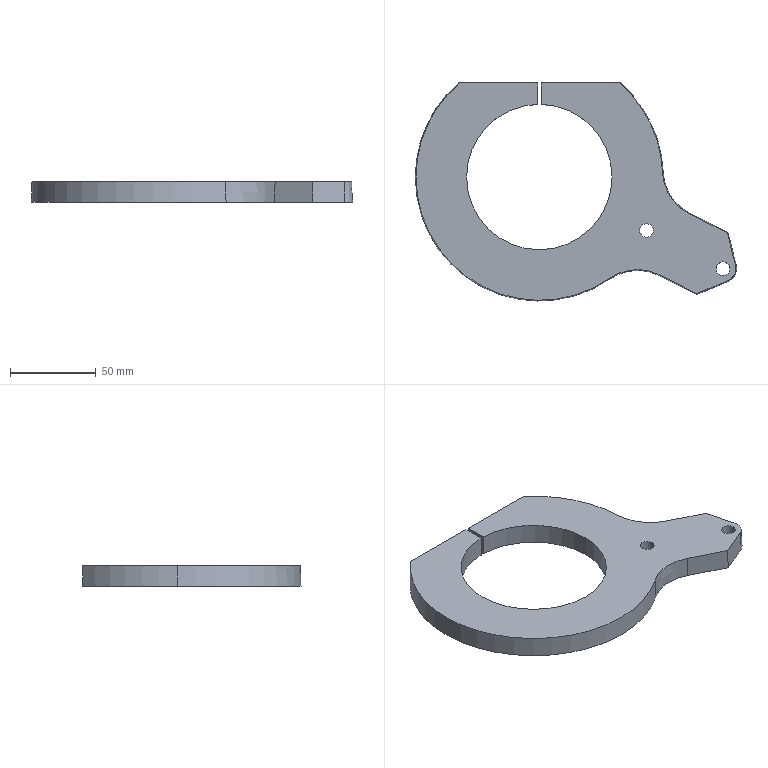Part | SolidWorks | features BaseBody 1 | 1 solid | 23 faces | box 187.892 x 127.5 x 12 mm | volume 139564 mm3 | plane 10 | cylinder 7 | cone 6 | commonest cylinder face diameters 8 x4 85 x3
STEP:
#1=CARTESIAN_POINT('',(-195.608,-53.544,12.));
#2=VERTEX_POINT('',#1);
#3=CARTESIAN_POINT('',(-187.608,-53.544,12.));
#4=VERTEX_POINT('',#3);
#5=CARTESIAN_POINT('',(-191.608,-53.544,12.));
#6=DIRECTION('',(0.,0.,1.));
#7=DIRECTION('',(-1.,0.,0.));
#8=AXIS2_PLACEMENT_3D('',#5,#6,#7);
#9=CIRCLE('',#8,4.);
#10=EDGE_CURVE('',#2,#4,#9,.T.);
#11=ORIENTED_EDGE('',*,*,#10,.T.);
#12=CARTESIAN_POINT('',(-187.608,-53.544,0.));
#13=VERTEX_POINT('',#12);
#14=CARTESIAN_POINT('',(-187.608,-53.544,12.));
#15=DIRECTION('',(0.,0.,-1.));
#16=VECTOR('',#15,1000.);
#17=LINE('',#14,#16);
#18=EDGE_CURVE('',#4,#13,#17,.T.);
#19=ORIENTED_EDGE('',*,*,#18,.T.);
#20=CARTESIAN_POINT('',(-195.608,-53.544,0.));
#21=VERTEX_POINT('',#20);
#22=CARTESIAN_POINT('',(-191.608,-53.544,0.));
#23=DIRECTION('',(0.,0.,-1.));
#24=DIRECTION('',(-1.,0.,0.));
#25=AXIS2_PLACEMENT_3D('',#22,#23,#24);
#26=CIRCLE('',#25,4.);
#27=EDGE_CURVE('',#13,#21,#26,.T.);
#28=ORIENTED_EDGE('',*,*,#27,.T.);
#29=CARTESIAN_POINT('',(-195.608,-53.544,12.));
#30=DIRECTION('',(0.,0.,-1.));
#31=VECTOR('',#30,1000.);
#32=LINE('',#29,#31);
#33=EDGE_CURVE('',#2,#21,#32,.T.);
#34=ORIENTED_EDGE('',*,*,#33,.F.);
#35=EDGE_LOOP('',(#11,#19,#28,#34));
#36=FACE_OUTER_BOUND('',#35,.T.);
#37=CARTESIAN_POINT('',(-191.608,-53.544,12.));
#38=DIRECTION('',(0.,0.,-1.));
#39=DIRECTION('',(-1.,0.,0.));
#40=AXIS2_PLACEMENT_3D('',#37,#38,#39);
#41=CYLINDRICAL_SURFACE('',#40,4.);
#42=ADVANCED_FACE('',(#36),#41,.F.);
#43=CARTESIAN_POINT('',(-232.355,-31.234,12.));
#44=VERTEX_POINT('',#43);
#45=CARTESIAN_POINT('',(-240.355,-31.234,12.));
#46=VERTEX_POINT('',#45);
#47=CARTESIAN_POINT('',(-236.355,-31.234,12.));
#48=DIRECTION('',(0.,0.,-1.));
#49=DIRECTION('',(-1.,0.,0.));
#50=AXIS2_PLACEMENT_3D('',#47,#48,#49);
#51=CIRCLE('',#50,4.);
#52=EDGE_CURVE('',#44,#46,#51,.T.);
#53=ORIENTED_EDGE('',*,*,#52,.F.);
#54=CARTESIAN_POINT('',(-232.355,-31.234,0.));
#55=VERTEX_POINT('',#54);
#56=CARTESIAN_POINT('',(-232.355,-31.234,12.));
#57=DIRECTION('',(0.,0.,-1.));
#58=VECTOR('',#57,1000.);
#59=LINE('',#56,#58);
#60=EDGE_CURVE('',#44,#55,#59,.T.);
#61=ORIENTED_EDGE('',*,*,#60,.T.);
#62=CARTESIAN_POINT('',(-240.355,-31.234,0.));
#63=VERTEX_POINT('',#62);
#64=CARTESIAN_POINT('',(-236.355,-31.234,0.));
#65=DIRECTION('',(0.,0.,-1.));
#66=DIRECTION('',(-1.,0.,0.));
#67=AXIS2_PLACEMENT_3D('',#64,#65,#66);
#68=CIRCLE('',#67,4.);
#69=EDGE_CURVE('',#55,#63,#68,.T.);
#70=ORIENTED_EDGE('',*,*,#69,.T.);
#71=CARTESIAN_POINT('',(-240.355,-31.234,12.));
#72=DIRECTION('',(0.,0.,-1.));
#73=VECTOR('',#72,1000.);
#74=LINE('',#71,#73);
#75=EDGE_CURVE('',#46,#63,#74,.T.);
#76=ORIENTED_EDGE('',*,*,#75,.F.);
#77=EDGE_LOOP('',(#53,#61,#70,#76));
#78=FACE_OUTER_BOUND('',#77,.T.);
#79=CARTESIAN_POINT('',(-236.355,-31.234,12.));
#80=DIRECTION('',(0.,0.,-1.));
#81=DIRECTION('',(-1.,0.,0.));
#82=AXIS2_PLACEMENT_3D('',#79,#80,#81);
#83=CYLINDRICAL_SURFACE('',#82,4.);
#84=ADVANCED_FACE('',(#78),#83,.F.);
#85=CARTESIAN_POINT('',(-371.081,0.,12.));
#86=VERTEX_POINT('',#85);
#87=CARTESIAN_POINT('',(-257.888,-59.207,12.));
#88=VERTEX_POINT('',#87);
#89=CARTESIAN_POINT('',(-299.,0.,12.));
#90=DIRECTION('',(0.,0.,1.));
#91=DIRECTION('',(-1.,0.,0.));
#92=AXIS2_PLACEMENT_3D('',#89,#90,#91);
#93=CIRCLE('',#92,72.081);
#94=EDGE_CURVE('',#86,#88,#93,.T.);
#95=ORIENTED_EDGE('',*,*,#94,.F.);
#96=CARTESIAN_POINT('',(-371.5,0.,0.));
#97=VERTEX_POINT('',#96);
#98=CARTESIAN_POINT('',(-371.081,0.,12.));
#99=DIRECTION('',(-0.0349,0.,-0.9994));
#100=VECTOR('',#99,1000.);
#101=LINE('',#98,#100);
#102=EDGE_CURVE('',#86,#97,#101,.T.);
#103=ORIENTED_EDGE('',*,*,#102,.T.);
#104=CARTESIAN_POINT('',(-257.649,-59.551,0.));
#105=VERTEX_POINT('',#104);
#106=CARTESIAN_POINT('',(-299.,0.,0.));
#107=DIRECTION('',(0.,0.,1.));
#108=DIRECTION('',(-1.,0.,0.));
#109=AXIS2_PLACEMENT_3D('',#106,#107,#108);
#110=CIRCLE('',#109,72.5);
#111=EDGE_CURVE('',#97,#105,#110,.T.);
#112=ORIENTED_EDGE('',*,*,#111,.T.);
#113=CARTESIAN_POINT('',(-257.768,-59.379,6.));
#114=DIRECTION('',(0.01991,-0.02867,-0.9994));
#115=VECTOR('',#114,1000.);
#116=LINE('',#113,#115);
#117=EDGE_CURVE('',#88,#105,#116,.T.);
#118=ORIENTED_EDGE('',*,*,#117,.F.);
#119=EDGE_LOOP('',(#95,#103,#112,#118));
#120=FACE_OUTER_BOUND('',#119,.T.);
#121=CARTESIAN_POINT('',(-299.,0.,12.));
#122=DIRECTION('',(0.,0.,-1.));
#123=DIRECTION('',(-1.,0.,0.));
#124=AXIS2_PLACEMENT_3D('',#121,#122,#123);
#125=CONICAL_SURFACE('',#124,72.081,0.03491);
#126=ADVANCED_FACE('',(#120),#125,.T.);
#127=CARTESIAN_POINT('',(-256.5,0.,12.));
#128=VERTEX_POINT('',#127);
#129=CARTESIAN_POINT('',(-341.5,0.,12.));
#130=VERTEX_POINT('',#129);
#131=CARTESIAN_POINT('',(-299.,0.,12.));
#132=DIRECTION('',(0.,0.,-1.));
#133=DIRECTION('',(-1.,0.,0.));
#134=AXIS2_PLACEMENT_3D('',#131,#132,#133);
#135=CIRCLE('',#134,42.5);
#136=EDGE_CURVE('',#128,#130,#135,.T.);
#137=ORIENTED_EDGE('',*,*,#136,.F.);
#138=CARTESIAN_POINT('',(-256.5,0.,0.));
#139=VERTEX_POINT('',#138);
#140=CARTESIAN_POINT('',(-256.5,0.,12.));
#141=DIRECTION('',(0.,0.,-1.));
#142=VECTOR('',#141,1000.);
#143=LINE('',#140,#142);
#144=EDGE_CURVE('',#128,#139,#143,.T.);
#145=ORIENTED_EDGE('',*,*,#144,.T.);
#146=CARTESIAN_POINT('',(-341.5,0.,0.));
#147=VERTEX_POINT('',#146);
#148=CARTESIAN_POINT('',(-299.,0.,0.));
#149=DIRECTION('',(0.,0.,-1.));
#150=DIRECTION('',(-1.,0.,0.));
#151=AXIS2_PLACEMENT_3D('',#148,#149,#150);
#152=CIRCLE('',#151,42.5);
#153=EDGE_CURVE('',#139,#147,#152,.T.);
#154=ORIENTED_EDGE('',*,*,#153,.T.);
#155=CARTESIAN_POINT('',(-341.5,0.,12.));
#156=DIRECTION('',(0.,0.,-1.));
#157=VECTOR('',#156,1000.);
#158=LINE('',#155,#157);
#159=EDGE_CURVE('',#130,#147,#158,.T.);
#160=ORIENTED_EDGE('',*,*,#159,.F.);
#161=EDGE_LOOP('',(#137,#145,#154,#160));
#162=FACE_OUTER_BOUND('',#161,.T.);
#163=CARTESIAN_POINT('',(-299.,0.,12.));
#164=DIRECTION('',(0.,0.,-1.));
#165=DIRECTION('',(-1.,0.,0.));
#166=AXIS2_PLACEMENT_3D('',#163,#164,#165);
#167=CYLINDRICAL_SURFACE('',#166,42.5);
#168=ADVANCED_FACE('',(#162),#167,.F.);
#169=CARTESIAN_POINT('',(-300.,42.488,12.));
#170=VERTEX_POINT('',#169);
#171=CARTESIAN_POINT('',(-299.,0.,12.));
#172=DIRECTION('',(0.,0.,-1.));
#173=DIRECTION('',(-1.,0.,0.));
#174=AXIS2_PLACEMENT_3D('',#171,#172,#173);
#175=CIRCLE('',#174,42.5);
#176=EDGE_CURVE('',#130,#170,#175,.T.);
#177=ORIENTED_EDGE('',*,*,#176,.F.);
#178=ORIENTED_EDGE('',*,*,#159,.T.);
#179=CARTESIAN_POINT('',(-300.,42.488,0.));
#180=VERTEX_POINT('',#179);
#181=CARTESIAN_POINT('',(-299.,0.,0.));
#182=DIRECTION('',(0.,0.,-1.));
#183=DIRECTION('',(-1.,0.,0.));
#184=AXIS2_PLACEMENT_3D('',#181,#182,#183);
#185=CIRCLE('',#184,42.5);
#186=EDGE_CURVE('',#147,#180,#185,.T.);
#187=ORIENTED_EDGE('',*,*,#186,.T.);
#188=CARTESIAN_POINT('',(-300.,42.488,6.));
#189=DIRECTION('',(0.,0.,1.));
#190=VECTOR('',#189,1000.);
#191=LINE('',#188,#190);
#192=EDGE_CURVE('',#180,#170,#191,.T.);
#193=ORIENTED_EDGE('',*,*,#192,.T.);
#194=EDGE_LOOP('',(#177,#178,#187,#193));
#195=FACE_OUTER_BOUND('',#194,.T.);
#196=CARTESIAN_POINT('',(-299.,0.,12.));
#197=DIRECTION('',(0.,0.,-1.));
#198=DIRECTION('',(-1.,0.,0.));
#199=AXIS2_PLACEMENT_3D('',#196,#197,#198);
#200=CYLINDRICAL_SURFACE('',#199,42.5);
#201=ADVANCED_FACE('',(#195),#200,.F.);
#202=ORIENTED_EDGE('',*,*,#18,.F.);
#203=CARTESIAN_POINT('',(-191.608,-53.544,12.));
#204=DIRECTION('',(0.,0.,1.));
#205=DIRECTION('',(-1.,0.,0.));
#206=AXIS2_PLACEMENT_3D('',#203,#204,#205);
#207=CIRCLE('',#206,4.);
#208=EDGE_CURVE('',#4,#2,#207,.T.);
#209=ORIENTED_EDGE('',*,*,#208,.T.);
#210=ORIENTED_EDGE('',*,*,#33,.T.);
#211=CARTESIAN_POINT('',(-191.608,-53.544,0.));
#212=DIRECTION('',(0.,0.,-1.));
#213=DIRECTION('',(-1.,0.,0.));
#214=AXIS2_PLACEMENT_3D('',#211,#212,#213);
#215=CIRCLE('',#214,4.);
#216=EDGE_CURVE('',#21,#13,#215,.T.);
#217=ORIENTED_EDGE('',*,*,#216,.T.);
#218=EDGE_LOOP('',(#202,#209,#210,#217));
#219=FACE_OUTER_BOUND('',#218,.T.);
#220=CARTESIAN_POINT('',(-191.608,-53.544,12.));
#221=DIRECTION('',(0.,0.,-1.));
#222=DIRECTION('',(-1.,0.,0.));
#223=AXIS2_PLACEMENT_3D('',#220,#221,#222);
#224=CYLINDRICAL_SURFACE('',#223,4.);
#225=ADVANCED_FACE('',(#219),#224,.F.);
#226=CARTESIAN_POINT('',(-236.355,-31.234,0.));
#227=DIRECTION('',(0.,0.,-1.));
#228=DIRECTION('',(-1.,0.,0.));
#229=AXIS2_PLACEMENT_3D('',#226,#227,#228);
#230=CIRCLE('',#229,4.);
#231=EDGE_CURVE('',#63,#55,#230,.T.);
#232=ORIENTED_EDGE('',*,*,#231,.F.);
#233=ORIENTED_EDGE('',*,*,#69,.F.);
#234=EDGE_LOOP('',(#232,#233));
#235=FACE_BOUND('',#234,.T.);
#236=ORIENTED_EDGE('',*,*,#216,.F.);
#237=ORIENTED_EDGE('',*,*,#27,.F.);
#238=EDGE_LOOP('',(#236,#237));
#239=FACE_BOUND('',#238,.T.);
#240=CARTESIAN_POINT('',(-211.069,-21.157,0.));
#241=VERTEX_POINT('',#240);
#242=CARTESIAN_POINT('',(-226.555,2.814,0.));
#243=VERTEX_POINT('',#242);
#244=CARTESIAN_POINT('',(-198.576,3.901,0.));
#245=DIRECTION('',(0.,0.,-1.));
#246=DIRECTION('',(1.,0.,0.));
#247=AXIS2_PLACEMENT_3D('',#244,#245,#246);
#248=CIRCLE('',#247,28.);
#249=EDGE_CURVE('',#241,#243,#248,.T.);
#250=ORIENTED_EDGE('',*,*,#249,.F.);
#251=CARTESIAN_POINT('',(-188.726,-32.297,0.));
#252=VERTEX_POINT('',#251);
#253=CARTESIAN_POINT('',(-211.069,-21.157,0.));
#254=DIRECTION('',(-0.8949,0.4462,0.));
#255=VECTOR('',#254,1000.);
#256=LINE('',#253,#255);
#257=EDGE_CURVE('',#252,#241,#256,.T.);
#258=ORIENTED_EDGE('',*,*,#257,.F.);
#259=CARTESIAN_POINT('',(-183.852,-51.583,-0.000000001));
#260=VERTEX_POINT('',#259);
#261=CARTESIAN_POINT('',(-188.756,-32.181,-0.000000003));
#262=DIRECTION('',(-0.245,0.9695,0.));
#263=VECTOR('',#262,1000.);
#264=LINE('',#261,#263);
#265=EDGE_CURVE('',#260,#252,#264,.T.);
#266=ORIENTED_EDGE('',*,*,#265,.F.);
#267=CARTESIAN_POINT('',(-188.506,-60.918,0.));
#268=VERTEX_POINT('',#267);
#269=CARTESIAN_POINT('',(-191.608,-53.544,0.));
#270=DIRECTION('',(0.,0.,1.));
#271=DIRECTION('',(-1.,0.,0.));
#272=AXIS2_PLACEMENT_3D('',#269,#270,#271);
#273=CIRCLE('',#272,8.);
#274=EDGE_CURVE('',#268,#260,#273,.T.);
#275=ORIENTED_EDGE('',*,*,#274,.F.);
#276=CARTESIAN_POINT('',(-206.842,-68.631,0.));
#277=VERTEX_POINT('',#276);
#278=CARTESIAN_POINT('',(-188.506,-60.918,0.));
#279=DIRECTION('',(0.9218,0.3878,0.));
#280=VECTOR('',#279,1000.);
#281=LINE('',#278,#280);
#282=EDGE_CURVE('',#277,#268,#281,.T.);
#283=ORIENTED_EDGE('',*,*,#282,.F.);
#284=CARTESIAN_POINT('',(-229.185,-57.492,0.));
#285=VERTEX_POINT('',#284);
#286=CARTESIAN_POINT('',(-206.708,-68.698,0.));
#287=DIRECTION('',(0.8949,-0.4462,0.));
#288=VECTOR('',#287,1000.);
#289=LINE('',#286,#288);
#290=EDGE_CURVE('',#285,#277,#289,.T.);
#291=ORIENTED_EDGE('',*,*,#290,.F.);
#292=CARTESIAN_POINT('',(-241.678,-82.55,0.));
#293=DIRECTION('',(0.,0.,-1.));
#294=DIRECTION('',(1.,0.,0.));
#295=AXIS2_PLACEMENT_3D('',#292,#293,#294);
#296=CIRCLE('',#295,28.);
#297=EDGE_CURVE('',#105,#285,#296,.T.);
#298=ORIENTED_EDGE('',*,*,#297,.F.);
#299=ORIENTED_EDGE('',*,*,#111,.F.);
#300=CARTESIAN_POINT('',(-346.236,55.,0.));
#301=VERTEX_POINT('',#300);
#302=CARTESIAN_POINT('',(-299.,0.,0.));
#303=DIRECTION('',(0.,0.,1.));
#304=DIRECTION('',(-1.,0.,0.));
#305=AXIS2_PLACEMENT_3D('',#302,#303,#304);
#306=CIRCLE('',#305,72.5);
#307=EDGE_CURVE('',#301,#97,#306,.T.);
#308=ORIENTED_EDGE('',*,*,#307,.F.);
#309=CARTESIAN_POINT('',(-300.,55.,0.));
#310=VERTEX_POINT('',#309);
#311=CARTESIAN_POINT('',(-277.554,55.,0.));
#312=DIRECTION('',(-1.,0.,0.));
#313=VECTOR('',#312,1000.);
#314=LINE('',#311,#313);
#315=EDGE_CURVE('',#310,#301,#314,.T.);
#316=ORIENTED_EDGE('',*,*,#315,.F.);
#317=CARTESIAN_POINT('',(-300.,-9.132,0.));
#318=DIRECTION('',(0.,1.,0.));
#319=VECTOR('',#318,1000.);
#320=LINE('',#317,#319);
#321=EDGE_CURVE('',#180,#310,#320,.T.);
#322=ORIENTED_EDGE('',*,*,#321,.F.);
#323=ORIENTED_EDGE('',*,*,#186,.F.);
#324=ORIENTED_EDGE('',*,*,#153,.F.);
#325=CARTESIAN_POINT('',(-298.,42.488,0.));
#326=VERTEX_POINT('',#325);
#327=CARTESIAN_POINT('',(-299.,0.,0.));
#328=DIRECTION('',(0.,0.,-1.));
#329=DIRECTION('',(-1.,0.,0.));
#330=AXIS2_PLACEMENT_3D('',#327,#328,#329);
#331=CIRCLE('',#330,42.5);
#332=EDGE_CURVE('',#326,#139,#331,.T.);
#333=ORIENTED_EDGE('',*,*,#332,.F.);
#334=CARTESIAN_POINT('',(-298.,55.,0.));
#335=VERTEX_POINT('',#334);
#336=CARTESIAN_POINT('',(-298.,-9.132,0.));
#337=DIRECTION('',(0.,-1.,0.));
#338=VECTOR('',#337,1000.);
#339=LINE('',#336,#338);
#340=EDGE_CURVE('',#335,#326,#339,.T.);
#341=ORIENTED_EDGE('',*,*,#340,.F.);
#342=CARTESIAN_POINT('',(-251.764,55.,0.));
#343=VERTEX_POINT('',#342);
#344=CARTESIAN_POINT('',(-277.554,55.,0.));
#345=DIRECTION('',(-1.,0.,0.));
#346=VECTOR('',#345,1000.);
#347=LINE('',#344,#346);
#348=EDGE_CURVE('',#343,#335,#347,.T.);
#349=ORIENTED_EDGE('',*,*,#348,.F.);
#350=CARTESIAN_POINT('',(-299.,0.,0.));
#351=DIRECTION('',(0.,0.,1.));
#352=DIRECTION('',(-1.,0.,0.));
#353=AXIS2_PLACEMENT_3D('',#350,#351,#352);
#354=CIRCLE('',#353,72.5);
#355=EDGE_CURVE('',#243,#343,#354,.T.);
#356=ORIENTED_EDGE('',*,*,#355,.F.);
#357=EDGE_LOOP('',(#250,#258,#266,#275,#283,#291,#298,#299,#308,#316,#322,#323,#324,#333,#341,#349,#356));
#358=FACE_OUTER_BOUND('',#357,.T.);
#359=CARTESIAN_POINT('',(-182.481,55.,0.));
#360=DIRECTION('',(0.,0.,1.));
#361=DIRECTION('',(-1.,0.,0.));
#362=AXIS2_PLACEMENT_3D('',#359,#360,#361);
#363=PLANE('',#362);
#364=ADVANCED_FACE('',(#235,#239,#358),#363,.F.);
#365=CARTESIAN_POINT('',(-236.355,-31.234,12.));
#366=DIRECTION('',(0.,0.,-1.));
#367=DIRECTION('',(-1.,0.,0.));
#368=AXIS2_PLACEMENT_3D('',#365,#366,#367);
#369=CIRCLE('',#368,4.);
#370=EDGE_CURVE('',#46,#44,#369,.T.);
#371=ORIENTED_EDGE('',*,*,#370,.T.);
#372=ORIENTED_EDGE('',*,*,#52,.T.);
#373=EDGE_LOOP('',(#371,#372));
#374=FACE_BOUND('',#373,.T.);
#375=ORIENTED_EDGE('',*,*,#10,.F.);
#376=ORIENTED_EDGE('',*,*,#208,.F.);
#377=EDGE_LOOP('',(#375,#376));
#378=FACE_BOUND('',#377,.T.);
#379=CARTESIAN_POINT('',(-211.256,-21.532,12.));
#380=VERTEX_POINT('',#379);
#381=CARTESIAN_POINT('',(-226.973,2.798,12.));
#382=VERTEX_POINT('',#381);
#383=CARTESIAN_POINT('',(-198.576,3.901,12.));
#384=DIRECTION('',(0.,0.,-1.));
#385=DIRECTION('',(1.,0.,0.));
#386=AXIS2_PLACEMENT_3D('',#383,#384,#385);
#387=CIRCLE('',#386,28.419);
#388=EDGE_CURVE('',#380,#382,#387,.T.);
#389=ORIENTED_EDGE('',*,*,#388,.T.);
#390=CARTESIAN_POINT('',(-252.41,55.,12.));
#391=VERTEX_POINT('',#390);
#392=CARTESIAN_POINT('',(-299.,0.,12.));
#393=DIRECTION('',(0.,0.,1.));
#394=DIRECTION('',(-1.,0.,0.));
#395=AXIS2_PLACEMENT_3D('',#392,#393,#394);
#396=CIRCLE('',#395,72.081);
#397=EDGE_CURVE('',#382,#391,#396,.T.);
#398=ORIENTED_EDGE('',*,*,#397,.T.);
#399=CARTESIAN_POINT('',(-298.,55.,12.));
#400=VERTEX_POINT('',#399);
#401=CARTESIAN_POINT('',(-277.554,55.,12.));
#402=DIRECTION('',(-1.,0.,0.));
#403=VECTOR('',#402,1000.);
#404=LINE('',#401,#403);
#405=EDGE_CURVE('',#391,#400,#404,.T.);
#406=ORIENTED_EDGE('',*,*,#405,.T.);
#407=CARTESIAN_POINT('',(-298.,42.488,12.));
#408=VERTEX_POINT('',#407);
#409=CARTESIAN_POINT('',(-298.,-8.922,12.));
#410=DIRECTION('',(0.,-1.,0.));
#411=VECTOR('',#410,1000.);
#412=LINE('',#409,#411);
#413=EDGE_CURVE('',#400,#408,#412,.T.);
#414=ORIENTED_EDGE('',*,*,#413,.T.);
#415=CARTESIAN_POINT('',(-299.,0.,12.));
#416=DIRECTION('',(0.,0.,-1.));
#417=DIRECTION('',(-1.,0.,0.));
#418=AXIS2_PLACEMENT_3D('',#415,#416,#417);
#419=CIRCLE('',#418,42.5);
#420=EDGE_CURVE('',#408,#128,#419,.T.);
#421=ORIENTED_EDGE('',*,*,#420,.T.);
#422=ORIENTED_EDGE('',*,*,#136,.T.);
#423=ORIENTED_EDGE('',*,*,#176,.T.);
#424=CARTESIAN_POINT('',(-300.,55.,12.));
#425=VERTEX_POINT('',#424);
#426=CARTESIAN_POINT('',(-300.,-8.922,12.));
#427=DIRECTION('',(0.,1.,0.));
#428=VECTOR('',#427,1000.);
#429=LINE('',#426,#428);
#430=EDGE_CURVE('',#170,#425,#429,.T.);
#431=ORIENTED_EDGE('',*,*,#430,.T.);
#432=CARTESIAN_POINT('',(-345.59,55.,12.));
#433=VERTEX_POINT('',#432);
#434=CARTESIAN_POINT('',(-277.554,55.,12.));
#435=DIRECTION('',(-1.,0.,0.));
#436=VECTOR('',#435,1000.);
#437=LINE('',#434,#436);
#438=EDGE_CURVE('',#425,#433,#437,.T.);
#439=ORIENTED_EDGE('',*,*,#438,.T.);
#440=CARTESIAN_POINT('',(-299.,0.,12.));
#441=DIRECTION('',(0.,0.,1.));
#442=DIRECTION('',(-1.,0.,0.));
#443=AXIS2_PLACEMENT_3D('',#440,#441,#442);
#444=CIRCLE('',#443,72.081);
#445=EDGE_CURVE('',#433,#86,#444,.T.);
#446=ORIENTED_EDGE('',*,*,#445,.T.);
#447=ORIENTED_EDGE('',*,*,#94,.T.);
#448=CARTESIAN_POINT('',(-228.998,-57.117,12.));
#449=VERTEX_POINT('',#448);
#450=CARTESIAN_POINT('',(-241.678,-82.55,12.));
#451=DIRECTION('',(0.,0.,-1.));
#452=DIRECTION('',(1.,0.,0.));
#453=AXIS2_PLACEMENT_3D('',#450,#451,#452);
#454=CIRCLE('',#453,28.419);
#455=EDGE_CURVE('',#88,#449,#454,.T.);
#456=ORIENTED_EDGE('',*,*,#455,.T.);
#457=CARTESIAN_POINT('',(-206.827,-68.171,12.));
#458=VERTEX_POINT('',#457);
#459=CARTESIAN_POINT('',(-228.998,-57.117,12.));
#460=DIRECTION('',(0.8949,-0.4462,0.));
#461=VECTOR('',#460,1000.);
#462=LINE('',#459,#461);
#463=EDGE_CURVE('',#449,#458,#462,.T.);
#464=ORIENTED_EDGE('',*,*,#463,.T.);
#465=CARTESIAN_POINT('',(-188.668,-60.532,12.));
#466=VERTEX_POINT('',#465);
#467=CARTESIAN_POINT('',(-206.827,-68.171,12.));
#468=DIRECTION('',(0.9218,0.3878,0.));
#469=VECTOR('',#468,1000.);
#470=LINE('',#467,#469);
#471=EDGE_CURVE('',#458,#466,#470,.T.);
#472=ORIENTED_EDGE('',*,*,#471,.T.);
#473=CARTESIAN_POINT('',(-184.258,-51.686,12.));
#474=VERTEX_POINT('',#473);
#475=CARTESIAN_POINT('',(-191.608,-53.544,12.));
#476=DIRECTION('',(0.,0.,1.));
#477=DIRECTION('',(-1.,0.,0.));
#478=AXIS2_PLACEMENT_3D('',#475,#476,#477);
#479=CIRCLE('',#478,7.581);
#480=EDGE_CURVE('',#466,#474,#479,.T.);
#481=ORIENTED_EDGE('',*,*,#480,.T.);
#482=CARTESIAN_POINT('',(-189.086,-32.586,12.));
#483=VERTEX_POINT('',#482);
#484=CARTESIAN_POINT('',(-184.258,-51.686,12.));
#485=DIRECTION('',(-0.245,0.9695,0.));
#486=VECTOR('',#485,1000.);
#487=LINE('',#484,#486);
#488=EDGE_CURVE('',#474,#483,#487,.T.);
#489=ORIENTED_EDGE('',*,*,#488,.T.);
#490=CARTESIAN_POINT('',(-189.086,-32.586,12.));
#491=DIRECTION('',(-0.8949,0.4462,0.));
#492=VECTOR('',#491,1000.);
#493=LINE('',#490,#492);
#494=EDGE_CURVE('',#483,#380,#493,.T.);
#495=ORIENTED_EDGE('',*,*,#494,.T.);
#496=EDGE_LOOP('',(#389,#398,#406,#414,#421,#422,#423,#431,#439,#446,#447,#456,#464,#472,#481,#489,#495));
#497=FACE_OUTER_BOUND('',#496,.T.);
#498=CARTESIAN_POINT('',(-182.905,55.,12.));
#499=DIRECTION('',(0.,0.,1.));
#500=DIRECTION('',(-1.,0.,0.));
#501=AXIS2_PLACEMENT_3D('',#498,#499,#500);
#502=PLANE('',#501);
#503=ADVANCED_FACE('',(#374,#378,#497),#502,.T.);
#504=ORIENTED_EDGE('',*,*,#60,.F.);
#505=ORIENTED_EDGE('',*,*,#370,.F.);
#506=ORIENTED_EDGE('',*,*,#75,.T.);
#507=ORIENTED_EDGE('',*,*,#231,.T.);
#508=EDGE_LOOP('',(#504,#505,#506,#507));
#509=FACE_OUTER_BOUND('',#508,.T.);
#510=CARTESIAN_POINT('',(-236.355,-31.234,12.));
#511=DIRECTION('',(0.,0.,-1.));
#512=DIRECTION('',(-1.,0.,0.));
#513=AXIS2_PLACEMENT_3D('',#510,#511,#512);
#514=CYLINDRICAL_SURFACE('',#513,4.);
#515=ADVANCED_FACE('',(#509),#514,.F.);
#516=CARTESIAN_POINT('',(-226.764,2.806,6.));
#517=DIRECTION('',(-0.03487,-0.001355,0.9994));
#518=VECTOR('',#517,1000.);
#519=LINE('',#516,#518);
#520=EDGE_CURVE('',#243,#382,#519,.T.);
#521=ORIENTED_EDGE('',*,*,#520,.F.);
#522=ORIENTED_EDGE('',*,*,#355,.T.);
#523=CARTESIAN_POINT('',(-252.41,55.,12.));
#524=CARTESIAN_POINT('',(-252.195,55.,8.028));
#525=CARTESIAN_POINT('',(-251.98,55.,4.028));
#526=CARTESIAN_POINT('',(-251.764,55.,0.));
#527=B_SPLINE_CURVE_WITH_KNOTS('',3,(#523,#524,#525,#526),.UNSPECIFIED.,.F.,.F.,(4,4),(0.,1.),.UNSPECIFIED.);
#528=EDGE_CURVE('',#391,#343,#527,.T.);
#529=ORIENTED_EDGE('',*,*,#528,.F.);
#530=ORIENTED_EDGE('',*,*,#397,.F.);
#531=EDGE_LOOP('',(#521,#522,#529,#530));
#532=FACE_OUTER_BOUND('',#531,.T.);
#533=CARTESIAN_POINT('',(-299.,0.,12.));
#534=DIRECTION('',(0.,0.,-1.));
#535=DIRECTION('',(-1.,0.,0.));
#536=AXIS2_PLACEMENT_3D('',#533,#534,#535);
#537=CONICAL_SURFACE('',#536,72.081,0.03491);
#538=ADVANCED_FACE('',(#532),#537,.T.);
#539=ORIENTED_EDGE('',*,*,#388,.F.);
#540=CARTESIAN_POINT('',(-211.163,-21.345,6.));
#541=DIRECTION('',(0.01557,0.03123,-0.9994));
#542=VECTOR('',#541,1000.);
#543=LINE('',#540,#542);
#544=EDGE_CURVE('',#380,#241,#543,.T.);
#545=ORIENTED_EDGE('',*,*,#544,.T.);
#546=ORIENTED_EDGE('',*,*,#249,.T.);
#547=ORIENTED_EDGE('',*,*,#520,.T.);
#548=EDGE_LOOP('',(#539,#545,#546,#547));
#549=FACE_OUTER_BOUND('',#548,.T.);
#550=CARTESIAN_POINT('',(-198.576,3.901,0.));
#551=DIRECTION('',(0.,0.,1.));
#552=DIRECTION('',(1.,0.,0.));
#553=AXIS2_PLACEMENT_3D('',#550,#551,#552);
#554=CONICAL_SURFACE('',#553,28.,0.03491);
#555=ADVANCED_FACE('',(#549),#554,.F.);
#556=ORIENTED_EDGE('',*,*,#494,.F.);
#557=CARTESIAN_POINT('',(-189.086,-32.586,12.));
#558=DIRECTION('',(0.02991,0.02408,-0.9993));
#559=VECTOR('',#558,1000.);
#560=LINE('',#557,#559);
#561=EDGE_CURVE('',#483,#252,#560,.T.);
#562=ORIENTED_EDGE('',*,*,#561,.T.);
#563=ORIENTED_EDGE('',*,*,#257,.T.);
#564=ORIENTED_EDGE('',*,*,#544,.F.);
#565=EDGE_LOOP('',(#556,#562,#563,#564));
#566=FACE_OUTER_BOUND('',#565,.T.);
#567=CARTESIAN_POINT('',(-211.256,-21.532,12.));
#568=DIRECTION('',(0.4459,0.8944,0.0349));
#569=DIRECTION('',(0.8949,-0.4462,0.));
#570=AXIS2_PLACEMENT_3D('',#567,#568,#569);
#571=PLANE('',#570);
#572=ADVANCED_FACE('',(#566),#571,.T.);
#573=ORIENTED_EDGE('',*,*,#488,.F.);
#574=CARTESIAN_POINT('',(-184.055,-51.635,6.));
#575=DIRECTION('',(0.03384,0.008552,-0.9994));
#576=VECTOR('',#575,1000.);
#577=LINE('',#574,#576);
#578=EDGE_CURVE('',#474,#260,#577,.T.);
#579=ORIENTED_EDGE('',*,*,#578,.T.);
#580=ORIENTED_EDGE('',*,*,#265,.T.);
#581=ORIENTED_EDGE('',*,*,#561,.F.);
#582=EDGE_LOOP('',(#573,#579,#580,#581));
#583=FACE_OUTER_BOUND('',#582,.T.);
#584=CARTESIAN_POINT('',(-189.162,-32.284,12.));
#585=DIRECTION('',(0.9689,0.2449,0.0349));
#586=DIRECTION('',(0.245,-0.9695,0.));
#587=AXIS2_PLACEMENT_3D('',#584,#585,#586);
#588=PLANE('',#587);
#589=ADVANCED_FACE('',(#583),#588,.T.);
#590=ORIENTED_EDGE('',*,*,#578,.F.);
#591=ORIENTED_EDGE('',*,*,#480,.F.);
#592=CARTESIAN_POINT('',(-188.587,-60.725,6.));
#593=DIRECTION('',(-0.01353,0.03217,0.9994));
#594=VECTOR('',#593,1000.);
#595=LINE('',#592,#594);
#596=EDGE_CURVE('',#268,#466,#595,.T.);
#597=ORIENTED_EDGE('',*,*,#596,.F.);
#598=ORIENTED_EDGE('',*,*,#274,.T.);
#599=EDGE_LOOP('',(#590,#591,#597,#598));
#600=FACE_OUTER_BOUND('',#599,.T.);
#601=CARTESIAN_POINT('',(-191.608,-53.544,12.));
#602=DIRECTION('',(0.,0.,-1.));
#603=DIRECTION('',(-1.,0.,0.));
#604=AXIS2_PLACEMENT_3D('',#601,#602,#603);
#605=CONICAL_SURFACE('',#604,7.581,0.03491);
#606=ADVANCED_FACE('',(#600),#605,.T.);
#607=ORIENTED_EDGE('',*,*,#471,.F.);
#608=CARTESIAN_POINT('',(-206.827,-68.171,12.));
#609=DIRECTION('',(-0.001234,-0.03838,-0.9993));
#610=VECTOR('',#609,1000.);
#611=LINE('',#608,#610);
#612=EDGE_CURVE('',#458,#277,#611,.T.);
#613=ORIENTED_EDGE('',*,*,#612,.T.);
#614=ORIENTED_EDGE('',*,*,#282,.T.);
#615=ORIENTED_EDGE('',*,*,#596,.T.);
#616=EDGE_LOOP('',(#607,#613,#614,#615));
#617=FACE_OUTER_BOUND('',#616,.T.);
#618=CARTESIAN_POINT('',(-188.668,-60.532,12.));
#619=DIRECTION('',(0.3875,-0.9212,0.0349));
#620=DIRECTION('',(-0.9218,-0.3878,0.));
#621=AXIS2_PLACEMENT_3D('',#618,#619,#620);
#622=PLANE('',#621);
#623=ADVANCED_FACE('',(#617),#622,.T.);
#624=ORIENTED_EDGE('',*,*,#463,.F.);
#625=CARTESIAN_POINT('',(-229.091,-57.304,6.));
#626=DIRECTION('',(-0.01557,-0.03123,-0.9994));
#627=VECTOR('',#626,1000.);
#628=LINE('',#625,#627);
#629=EDGE_CURVE('',#449,#285,#628,.T.);
#630=ORIENTED_EDGE('',*,*,#629,.T.);
#631=ORIENTED_EDGE('',*,*,#290,.T.);
#632=ORIENTED_EDGE('',*,*,#612,.F.);
#633=EDGE_LOOP('',(#624,#630,#631,#632));
#634=FACE_OUTER_BOUND('',#633,.T.);
#635=CARTESIAN_POINT('',(-206.521,-68.323,12.));
#636=DIRECTION('',(-0.4459,-0.8944,0.0349));
#637=DIRECTION('',(-0.8949,0.4462,0.));
#638=AXIS2_PLACEMENT_3D('',#635,#636,#637);
#639=PLANE('',#638);
#640=ADVANCED_FACE('',(#634),#639,.T.);
#641=ORIENTED_EDGE('',*,*,#455,.F.);
#642=ORIENTED_EDGE('',*,*,#117,.T.);
#643=ORIENTED_EDGE('',*,*,#297,.T.);
#644=ORIENTED_EDGE('',*,*,#629,.F.);
#645=EDGE_LOOP('',(#641,#642,#643,#644));
#646=FACE_OUTER_BOUND('',#645,.T.);
#647=CARTESIAN_POINT('',(-241.678,-82.55,0.));
#648=DIRECTION('',(0.,0.,1.));
#649=DIRECTION('',(1.,0.,0.));
#650=AXIS2_PLACEMENT_3D('',#647,#648,#649);
#651=CONICAL_SURFACE('',#650,28.,0.03491);
#652=ADVANCED_FACE('',(#646),#651,.F.);
#653=ORIENTED_EDGE('',*,*,#102,.F.);
#654=ORIENTED_EDGE('',*,*,#445,.F.);
#655=CARTESIAN_POINT('',(-346.236,55.,0.));
#656=CARTESIAN_POINT('',(-346.02,55.,4.028));
#657=CARTESIAN_POINT('',(-345.805,55.,8.028));
#658=CARTESIAN_POINT('',(-345.59,55.,12.));
#659=B_SPLINE_CURVE_WITH_KNOTS('',3,(#655,#656,#657,#658),.UNSPECIFIED.,.F.,.F.,(4,4),(0.,1.),.UNSPECIFIED.);
#660=EDGE_CURVE('',#301,#433,#659,.T.);
#661=ORIENTED_EDGE('',*,*,#660,.F.);
#662=ORIENTED_EDGE('',*,*,#307,.T.);
#663=EDGE_LOOP('',(#653,#654,#661,#662));
#664=FACE_OUTER_BOUND('',#663,.T.);
#665=CARTESIAN_POINT('',(-299.,0.,12.));
#666=DIRECTION('',(0.,0.,-1.));
#667=DIRECTION('',(-1.,0.,0.));
#668=AXIS2_PLACEMENT_3D('',#665,#666,#667);
#669=CONICAL_SURFACE('',#668,72.081,0.03491);
#670=ADVANCED_FACE('',(#664),#669,.T.);
#671=ORIENTED_EDGE('',*,*,#660,.T.);
#672=ORIENTED_EDGE('',*,*,#438,.F.);
#673=CARTESIAN_POINT('',(-300.,55.,6.));
#674=DIRECTION('',(0.,0.,1.));
#675=VECTOR('',#674,1000.);
#676=LINE('',#673,#675);
#677=EDGE_CURVE('',#310,#425,#676,.T.);
#678=ORIENTED_EDGE('',*,*,#677,.F.);
#679=ORIENTED_EDGE('',*,*,#315,.T.);
#680=EDGE_LOOP('',(#671,#672,#678,#679));
#681=FACE_OUTER_BOUND('',#680,.T.);
#682=CARTESIAN_POINT('',(-346.514,55.,12.));
#683=DIRECTION('',(0.,-1.,0.));
#684=DIRECTION('',(0.,0.,-1.));
#685=AXIS2_PLACEMENT_3D('',#682,#683,#684);
#686=PLANE('',#685);
#687=ADVANCED_FACE('',(#681),#686,.F.);
#688=ORIENTED_EDGE('',*,*,#192,.F.);
#689=ORIENTED_EDGE('',*,*,#321,.T.);
#690=ORIENTED_EDGE('',*,*,#677,.T.);
#691=ORIENTED_EDGE('',*,*,#430,.F.);
#692=EDGE_LOOP('',(#688,#689,#690,#691));
#693=FACE_OUTER_BOUND('',#692,.T.);
#694=CARTESIAN_POINT('',(-300.,42.488,12.));
#695=DIRECTION('',(-1.,0.,0.));
#696=DIRECTION('',(0.,1.,0.));
#697=AXIS2_PLACEMENT_3D('',#694,#695,#696);
#698=PLANE('',#697);
#699=ADVANCED_FACE('',(#693),#698,.F.);
#700=ORIENTED_EDGE('',*,*,#144,.F.);
#701=ORIENTED_EDGE('',*,*,#420,.F.);
#702=CARTESIAN_POINT('',(-298.,42.488,6.));
#703=DIRECTION('',(0.,0.,-1.));
#704=VECTOR('',#703,1000.);
#705=LINE('',#702,#704);
#706=EDGE_CURVE('',#408,#326,#705,.T.);
#707=ORIENTED_EDGE('',*,*,#706,.T.);
#708=ORIENTED_EDGE('',*,*,#332,.T.);
#709=EDGE_LOOP('',(#700,#701,#707,#708));
#710=FACE_OUTER_BOUND('',#709,.T.);
#711=CARTESIAN_POINT('',(-299.,0.,12.));
#712=DIRECTION('',(0.,0.,-1.));
#713=DIRECTION('',(-1.,0.,0.));
#714=AXIS2_PLACEMENT_3D('',#711,#712,#713);
#715=CYLINDRICAL_SURFACE('',#714,42.5);
#716=ADVANCED_FACE('',(#710),#715,.F.);
#717=CARTESIAN_POINT('',(-298.,55.,6.));
#718=DIRECTION('',(0.,0.,1.));
#719=VECTOR('',#718,1000.);
#720=LINE('',#717,#719);
#721=EDGE_CURVE('',#335,#400,#720,.T.);
#722=ORIENTED_EDGE('',*,*,#721,.F.);
#723=ORIENTED_EDGE('',*,*,#340,.T.);
#724=ORIENTED_EDGE('',*,*,#706,.F.);
#725=ORIENTED_EDGE('',*,*,#413,.F.);
#726=EDGE_LOOP('',(#722,#723,#724,#725));
#727=FACE_OUTER_BOUND('',#726,.T.);
#728=CARTESIAN_POINT('',(-298.,55.,12.));
#729=DIRECTION('',(1.,0.,0.));
#730=DIRECTION('',(0.,-1.,0.));
#731=AXIS2_PLACEMENT_3D('',#728,#729,#730);
#732=PLANE('',#731);
#733=ADVANCED_FACE('',(#727),#732,.F.);
#734=ORIENTED_EDGE('',*,*,#528,.T.);
#735=ORIENTED_EDGE('',*,*,#348,.T.);
#736=ORIENTED_EDGE('',*,*,#721,.T.);
#737=ORIENTED_EDGE('',*,*,#405,.F.);
#738=EDGE_LOOP('',(#734,#735,#736,#737));
#739=FACE_OUTER_BOUND('',#738,.T.);
#740=CARTESIAN_POINT('',(-298.,55.,12.));
#741=DIRECTION('',(0.,-1.,0.));
#742=DIRECTION('',(0.,0.,-1.));
#743=AXIS2_PLACEMENT_3D('',#740,#741,#742);
#744=PLANE('',#743);
#745=ADVANCED_FACE('',(#739),#744,.F.);
#746=CLOSED_SHELL('',(#42,#84,#126,#168,#201,#225,#364,#503,#515,#538,#555,#572,#589,#606,#623,#640,#652,#670,#687,#699,#716,#733,#745));
#747=MANIFOLD_SOLID_BREP('',#746);
#748=CARTESIAN_POINT('',(0.,0.,0.));
#749=DIRECTION('',(0.,0.,1.));
#750=DIRECTION('',(1.,0.,0.));
#751=AXIS2_PLACEMENT_3D('',#748,#749,#750);
#752=(LENGTH_UNIT()NAMED_UNIT(*)SI_UNIT(.MILLI.,.METRE.));
#753=UNCERTAINTY_MEASURE_WITH_UNIT(LENGTH_MEASURE(0.00001),#752,'','');
#754=(NAMED_UNIT(*)PLANE_ANGLE_UNIT()SI_UNIT($,.RADIAN.));
#755=(NAMED_UNIT(*)SI_UNIT($,.STERADIAN.)SOLID_ANGLE_UNIT());
#756=(GEOMETRIC_REPRESENTATION_CONTEXT(3)GLOBAL_UNCERTAINTY_ASSIGNED_CONTEXT((#753))GLOBAL_UNIT_ASSIGNED_CONTEXT((#752,#754,#755))REPRESENTATION_CONTEXT('',''));
#757=ADVANCED_BREP_SHAPE_REPRESENTATION('',(#747,#751),#756);